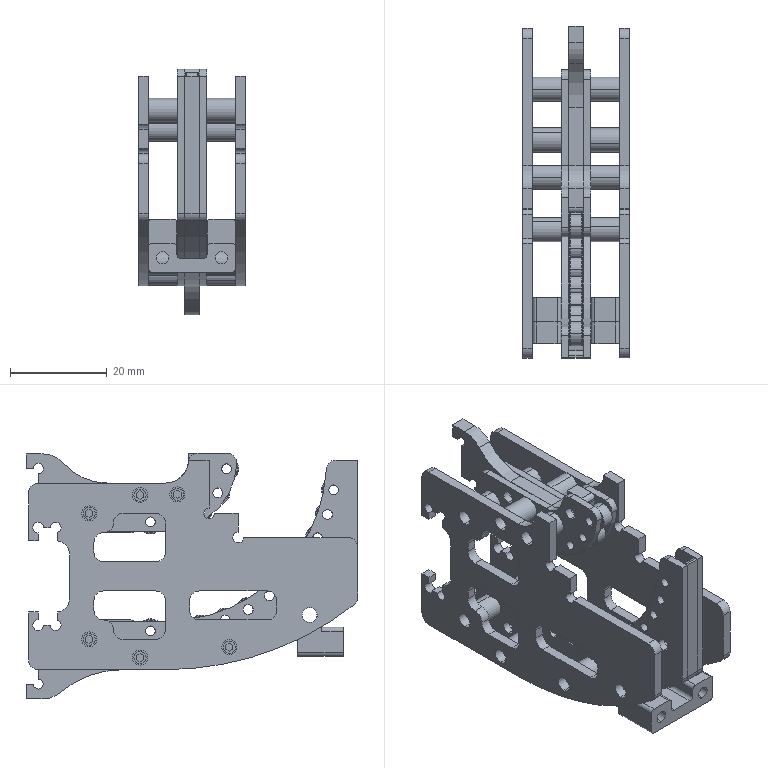Part | SolidWorks | features CompositeCurve 1 | 43 solids | 1007 faces | box 22 x 68.45 x 50.65 mm | volume 15273 mm3 | cylinder 554 | plane 313 | torus 128 | cone 12 | commonest cylinder face diameters 3.1 x70 2.05 x64 2.7 x64 4.4 x64 4 x60 5 x56